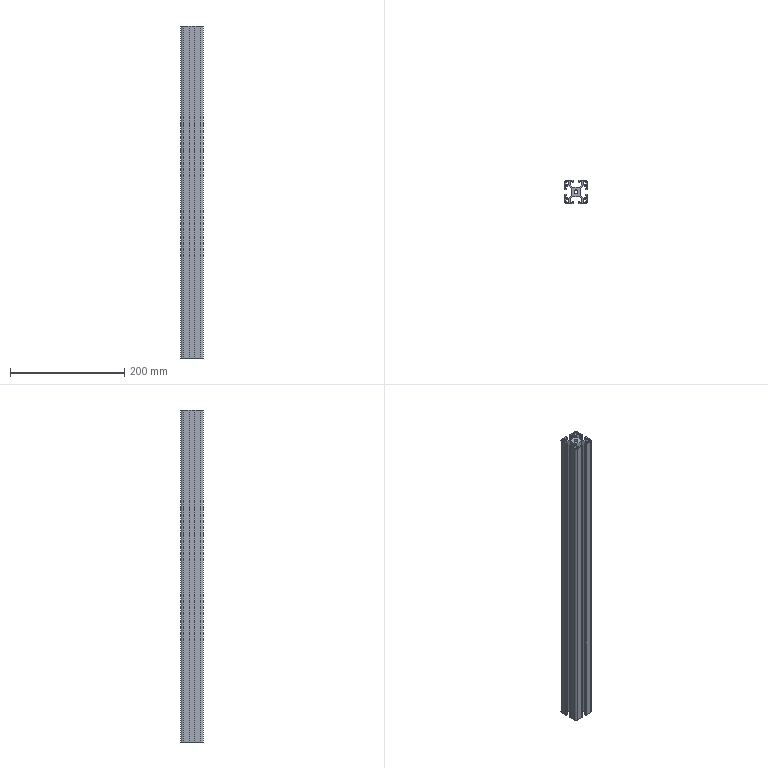Part | NX | features DATUM_CSYS 2, EXTRUDE 1, SKETCH 1 | 1 solid | 103 faces | box 40 x 40 x 580 mm | volume 334396 mm3 | plane 94 | cylinder 9 | commonest cylinder face diameters 5 x4 9 x4 6.8 x1